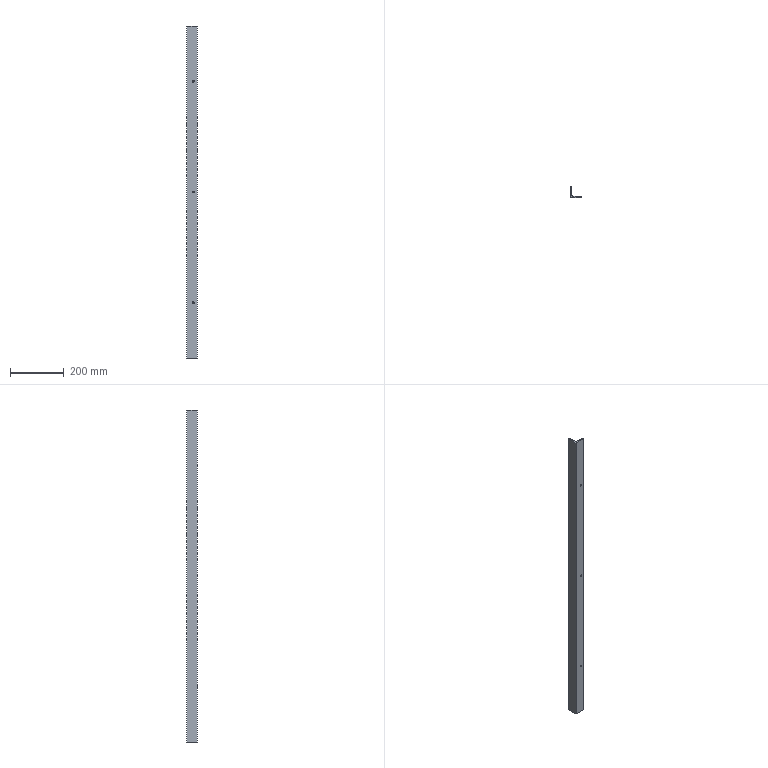Part | SolidWorks | features Extrusion 1, HoleWzd 1, LPattern 1 | 1 solid | 17 faces | box 40 x 40 x 1230 mm | volume 378926 mm3 | cylinder 9 | plane 8 | commonest cylinder face diameters 6 x6 0.02 x2 9 x1
STEP:
#1=CARTESIAN_POINT('',(25.,4.,1028.));
#2=VERTEX_POINT('',#1);
#3=CARTESIAN_POINT('',(25.,4.,1022.));
#4=VERTEX_POINT('',#3);
#5=CARTESIAN_POINT('',(25.,4.,1025.));
#6=DIRECTION('',(0.,-1.,0.));
#7=DIRECTION('',(1.,0.,0.));
#8=AXIS2_PLACEMENT_3D('',#5,#6,#7);
#9=CIRCLE('',#8,3.);
#10=EDGE_CURVE('',#2,#4,#9,.T.);
#11=ORIENTED_EDGE('',*,*,#10,.F.);
#12=CARTESIAN_POINT('',(25.,0.,1028.));
#13=VERTEX_POINT('',#12);
#14=CARTESIAN_POINT('',(25.,0.,1028.));
#15=DIRECTION('',(0.,-1.,0.));
#16=VECTOR('',#15,1000.);
#17=LINE('',#14,#16);
#18=EDGE_CURVE('',#2,#13,#17,.T.);
#19=ORIENTED_EDGE('',*,*,#18,.T.);
#20=CARTESIAN_POINT('',(25.,0.,1022.));
#21=VERTEX_POINT('',#20);
#22=CARTESIAN_POINT('',(25.,0.,1025.));
#23=DIRECTION('',(0.,-1.,0.));
#24=DIRECTION('',(0.,0.,-1.));
#25=AXIS2_PLACEMENT_3D('',#22,#23,#24);
#26=CIRCLE('',#25,3.);
#27=EDGE_CURVE('',#13,#21,#26,.T.);
#28=ORIENTED_EDGE('',*,*,#27,.T.);
#29=CARTESIAN_POINT('',(25.,0.,1022.));
#30=DIRECTION('',(0.,-1.,0.));
#31=VECTOR('',#30,1000.);
#32=LINE('',#29,#31);
#33=EDGE_CURVE('',#4,#21,#32,.T.);
#34=ORIENTED_EDGE('',*,*,#33,.F.);
#35=EDGE_LOOP('',(#11,#19,#28,#34));
#36=FACE_OUTER_BOUND('',#35,.T.);
#37=CARTESIAN_POINT('',(25.,0.,1025.));
#38=DIRECTION('',(0.,-1.,0.));
#39=DIRECTION('',(0.,0.,-1.));
#40=AXIS2_PLACEMENT_3D('',#37,#38,#39);
#41=CYLINDRICAL_SURFACE('',#40,3.);
#42=ADVANCED_FACE('',(#36),#41,.F.);
#43=CARTESIAN_POINT('',(25.,4.,618.));
#44=VERTEX_POINT('',#43);
#45=CARTESIAN_POINT('',(25.,4.,612.));
#46=VERTEX_POINT('',#45);
#47=CARTESIAN_POINT('',(25.,4.,615.));
#48=DIRECTION('',(0.,-1.,0.));
#49=DIRECTION('',(1.,0.,0.));
#50=AXIS2_PLACEMENT_3D('',#47,#48,#49);
#51=CIRCLE('',#50,3.);
#52=EDGE_CURVE('',#44,#46,#51,.T.);
#53=ORIENTED_EDGE('',*,*,#52,.F.);
#54=CARTESIAN_POINT('',(25.,0.,618.));
#55=VERTEX_POINT('',#54);
#56=CARTESIAN_POINT('',(25.,0.,618.));
#57=DIRECTION('',(0.,-1.,0.));
#58=VECTOR('',#57,1000.);
#59=LINE('',#56,#58);
#60=EDGE_CURVE('',#44,#55,#59,.T.);
#61=ORIENTED_EDGE('',*,*,#60,.T.);
#62=CARTESIAN_POINT('',(25.,0.,612.));
#63=VERTEX_POINT('',#62);
#64=CARTESIAN_POINT('',(25.,0.,615.));
#65=DIRECTION('',(0.,-1.,0.));
#66=DIRECTION('',(0.,0.,-1.));
#67=AXIS2_PLACEMENT_3D('',#64,#65,#66);
#68=CIRCLE('',#67,3.);
#69=EDGE_CURVE('',#55,#63,#68,.T.);
#70=ORIENTED_EDGE('',*,*,#69,.T.);
#71=CARTESIAN_POINT('',(25.,0.,612.));
#72=DIRECTION('',(0.,-1.,0.));
#73=VECTOR('',#72,1000.);
#74=LINE('',#71,#73);
#75=EDGE_CURVE('',#46,#63,#74,.T.);
#76=ORIENTED_EDGE('',*,*,#75,.F.);
#77=EDGE_LOOP('',(#53,#61,#70,#76));
#78=FACE_OUTER_BOUND('',#77,.T.);
#79=CARTESIAN_POINT('',(25.,0.,615.));
#80=DIRECTION('',(0.,-1.,0.));
#81=DIRECTION('',(0.,0.,-1.));
#82=AXIS2_PLACEMENT_3D('',#79,#80,#81);
#83=CYLINDRICAL_SURFACE('',#82,3.);
#84=ADVANCED_FACE('',(#78),#83,.F.);
#85=CARTESIAN_POINT('',(25.,4.,208.));
#86=VERTEX_POINT('',#85);
#87=CARTESIAN_POINT('',(25.,4.,202.));
#88=VERTEX_POINT('',#87);
#89=CARTESIAN_POINT('',(25.,4.,205.));
#90=DIRECTION('',(0.,-1.,0.));
#91=DIRECTION('',(1.,0.,0.));
#92=AXIS2_PLACEMENT_3D('',#89,#90,#91);
#93=CIRCLE('',#92,3.);
#94=EDGE_CURVE('',#86,#88,#93,.T.);
#95=ORIENTED_EDGE('',*,*,#94,.F.);
#96=CARTESIAN_POINT('',(25.,0.,208.));
#97=VERTEX_POINT('',#96);
#98=CARTESIAN_POINT('',(25.,0.,208.));
#99=DIRECTION('',(0.,-1.,0.));
#100=VECTOR('',#99,1000.);
#101=LINE('',#98,#100);
#102=EDGE_CURVE('',#86,#97,#101,.T.);
#103=ORIENTED_EDGE('',*,*,#102,.T.);
#104=CARTESIAN_POINT('',(25.,0.,202.));
#105=VERTEX_POINT('',#104);
#106=CARTESIAN_POINT('',(25.,0.,205.));
#107=DIRECTION('',(0.,-1.,0.));
#108=DIRECTION('',(0.,0.,-1.));
#109=AXIS2_PLACEMENT_3D('',#106,#107,#108);
#110=CIRCLE('',#109,3.);
#111=EDGE_CURVE('',#97,#105,#110,.T.);
#112=ORIENTED_EDGE('',*,*,#111,.T.);
#113=CARTESIAN_POINT('',(25.,0.,202.));
#114=DIRECTION('',(0.,-1.,0.));
#115=VECTOR('',#114,1000.);
#116=LINE('',#113,#115);
#117=EDGE_CURVE('',#88,#105,#116,.T.);
#118=ORIENTED_EDGE('',*,*,#117,.F.);
#119=EDGE_LOOP('',(#95,#103,#112,#118));
#120=FACE_OUTER_BOUND('',#119,.T.);
#121=CARTESIAN_POINT('',(25.,0.,205.));
#122=DIRECTION('',(0.,-1.,0.));
#123=DIRECTION('',(0.,0.,-1.));
#124=AXIS2_PLACEMENT_3D('',#121,#122,#123);
#125=CYLINDRICAL_SURFACE('',#124,3.);
#126=ADVANCED_FACE('',(#120),#125,.F.);
#127=CARTESIAN_POINT('',(25.,0.,615.));
#128=DIRECTION('',(0.,-1.,0.));
#129=DIRECTION('',(0.,0.,-1.));
#130=AXIS2_PLACEMENT_3D('',#127,#128,#129);
#131=CIRCLE('',#130,3.);
#132=EDGE_CURVE('',#63,#55,#131,.T.);
#133=ORIENTED_EDGE('',*,*,#132,.F.);
#134=ORIENTED_EDGE('',*,*,#69,.F.);
#135=EDGE_LOOP('',(#133,#134));
#136=FACE_BOUND('',#135,.T.);
#137=CARTESIAN_POINT('',(25.,0.,205.));
#138=DIRECTION('',(0.,-1.,0.));
#139=DIRECTION('',(0.,0.,-1.));
#140=AXIS2_PLACEMENT_3D('',#137,#138,#139);
#141=CIRCLE('',#140,3.);
#142=EDGE_CURVE('',#105,#97,#141,.T.);
#143=ORIENTED_EDGE('',*,*,#142,.F.);
#144=ORIENTED_EDGE('',*,*,#111,.F.);
#145=EDGE_LOOP('',(#143,#144));
#146=FACE_BOUND('',#145,.T.);
#147=CARTESIAN_POINT('',(0.,0.,0.));
#148=VERTEX_POINT('',#147);
#149=CARTESIAN_POINT('',(40.,0.,0.));
#150=VERTEX_POINT('',#149);
#151=CARTESIAN_POINT('',(40.,0.,0.));
#152=DIRECTION('',(1.,0.,0.));
#153=VECTOR('',#152,1000.);
#154=LINE('',#151,#153);
#155=EDGE_CURVE('',#148,#150,#154,.T.);
#156=ORIENTED_EDGE('',*,*,#155,.T.);
#157=CARTESIAN_POINT('',(40.,0.,1230.));
#158=VERTEX_POINT('',#157);
#159=CARTESIAN_POINT('',(40.,0.,1230.));
#160=DIRECTION('',(0.,0.,-1.));
#161=VECTOR('',#160,1000.);
#162=LINE('',#159,#161);
#163=EDGE_CURVE('',#158,#150,#162,.T.);
#164=ORIENTED_EDGE('',*,*,#163,.F.);
#165=CARTESIAN_POINT('',(0.,0.,1230.));
#166=VERTEX_POINT('',#165);
#167=CARTESIAN_POINT('',(40.,0.,1230.));
#168=DIRECTION('',(1.,0.,0.));
#169=VECTOR('',#168,1000.);
#170=LINE('',#167,#169);
#171=EDGE_CURVE('',#166,#158,#170,.T.);
#172=ORIENTED_EDGE('',*,*,#171,.F.);
#173=CARTESIAN_POINT('',(0.,0.,1230.));
#174=DIRECTION('',(0.,0.,-1.));
#175=VECTOR('',#174,1000.);
#176=LINE('',#173,#175);
#177=EDGE_CURVE('',#166,#148,#176,.T.);
#178=ORIENTED_EDGE('',*,*,#177,.T.);
#179=EDGE_LOOP('',(#156,#164,#172,#178));
#180=FACE_OUTER_BOUND('',#179,.T.);
#181=CARTESIAN_POINT('',(25.,0.,1025.));
#182=DIRECTION('',(0.,-1.,0.));
#183=DIRECTION('',(0.,0.,-1.));
#184=AXIS2_PLACEMENT_3D('',#181,#182,#183);
#185=CIRCLE('',#184,3.);
#186=EDGE_CURVE('',#21,#13,#185,.T.);
#187=ORIENTED_EDGE('',*,*,#186,.F.);
#188=ORIENTED_EDGE('',*,*,#27,.F.);
#189=EDGE_LOOP('',(#187,#188));
#190=FACE_BOUND('',#189,.T.);
#191=CARTESIAN_POINT('',(40.,0.,1230.));
#192=DIRECTION('',(0.,1.,0.));
#193=DIRECTION('',(-1.,0.,0.));
#194=AXIS2_PLACEMENT_3D('',#191,#192,#193);
#195=PLANE('',#194);
#196=ADVANCED_FACE('',(#136,#146,#180,#190),#195,.F.);
#197=CARTESIAN_POINT('',(40.,3.99,0.));
#198=VERTEX_POINT('',#197);
#199=CARTESIAN_POINT('',(40.,3.99,0.));
#200=DIRECTION('',(0.,1.,0.));
#201=VECTOR('',#200,1000.);
#202=LINE('',#199,#201);
#203=EDGE_CURVE('',#150,#198,#202,.T.);
#204=ORIENTED_EDGE('',*,*,#203,.T.);
#205=CARTESIAN_POINT('',(40.,3.99,1230.));
#206=VERTEX_POINT('',#205);
#207=CARTESIAN_POINT('',(40.,3.99,1230.));
#208=DIRECTION('',(0.,0.,-1.));
#209=VECTOR('',#208,1000.);
#210=LINE('',#207,#209);
#211=EDGE_CURVE('',#206,#198,#210,.T.);
#212=ORIENTED_EDGE('',*,*,#211,.F.);
#213=CARTESIAN_POINT('',(40.,3.99,1230.));
#214=DIRECTION('',(0.,1.,0.));
#215=VECTOR('',#214,1000.);
#216=LINE('',#213,#215);
#217=EDGE_CURVE('',#158,#206,#216,.T.);
#218=ORIENTED_EDGE('',*,*,#217,.F.);
#219=ORIENTED_EDGE('',*,*,#163,.T.);
#220=EDGE_LOOP('',(#204,#212,#218,#219));
#221=FACE_OUTER_BOUND('',#220,.T.);
#222=CARTESIAN_POINT('',(40.,3.99,1230.));
#223=DIRECTION('',(-1.,0.,0.));
#224=DIRECTION('',(0.,0.,1.));
#225=AXIS2_PLACEMENT_3D('',#222,#223,#224);
#226=PLANE('',#225);
#227=ADVANCED_FACE('',(#221),#226,.F.);
#228=CARTESIAN_POINT('',(39.99,4.,0.));
#229=VERTEX_POINT('',#228);
#230=CARTESIAN_POINT('',(39.99,3.99,0.));
#231=DIRECTION('',(0.,0.,1.));
#232=DIRECTION('',(1.,0.,0.));
#233=AXIS2_PLACEMENT_3D('',#230,#231,#232);
#234=CIRCLE('',#233,0.01);
#235=EDGE_CURVE('',#198,#229,#234,.T.);
#236=ORIENTED_EDGE('',*,*,#235,.T.);
#237=CARTESIAN_POINT('',(39.99,4.,1230.));
#238=VERTEX_POINT('',#237);
#239=CARTESIAN_POINT('',(39.99,4.,1230.));
#240=DIRECTION('',(0.,0.,-1.));
#241=VECTOR('',#240,1000.);
#242=LINE('',#239,#241);
#243=EDGE_CURVE('',#238,#229,#242,.T.);
#244=ORIENTED_EDGE('',*,*,#243,.F.);
#245=CARTESIAN_POINT('',(39.99,3.99,1230.));
#246=DIRECTION('',(0.,0.,1.));
#247=DIRECTION('',(1.,0.,0.));
#248=AXIS2_PLACEMENT_3D('',#245,#246,#247);
#249=CIRCLE('',#248,0.01);
#250=EDGE_CURVE('',#206,#238,#249,.T.);
#251=ORIENTED_EDGE('',*,*,#250,.F.);
#252=ORIENTED_EDGE('',*,*,#211,.T.);
#253=EDGE_LOOP('',(#236,#244,#251,#252));
#254=FACE_OUTER_BOUND('',#253,.T.);
#255=CARTESIAN_POINT('',(39.99,3.99,1230.));
#256=DIRECTION('',(0.,0.,-1.));
#257=DIRECTION('',(-1.,0.,0.));
#258=AXIS2_PLACEMENT_3D('',#255,#256,#257);
#259=CYLINDRICAL_SURFACE('',#258,0.01);
#260=ADVANCED_FACE('',(#254),#259,.T.);
#261=CARTESIAN_POINT('',(25.,4.,615.));
#262=DIRECTION('',(0.,-1.,0.));
#263=DIRECTION('',(1.,0.,0.));
#264=AXIS2_PLACEMENT_3D('',#261,#262,#263);
#265=CIRCLE('',#264,3.);
#266=EDGE_CURVE('',#46,#44,#265,.T.);
#267=ORIENTED_EDGE('',*,*,#266,.T.);
#268=ORIENTED_EDGE('',*,*,#52,.T.);
#269=EDGE_LOOP('',(#267,#268));
#270=FACE_BOUND('',#269,.T.);
#271=CARTESIAN_POINT('',(25.,4.,205.));
#272=DIRECTION('',(0.,-1.,0.));
#273=DIRECTION('',(1.,0.,0.));
#274=AXIS2_PLACEMENT_3D('',#271,#272,#273);
#275=CIRCLE('',#274,3.);
#276=EDGE_CURVE('',#88,#86,#275,.T.);
#277=ORIENTED_EDGE('',*,*,#276,.T.);
#278=ORIENTED_EDGE('',*,*,#94,.T.);
#279=EDGE_LOOP('',(#277,#278));
#280=FACE_BOUND('',#279,.T.);
#281=CARTESIAN_POINT('',(8.5,4.,0.));
#282=VERTEX_POINT('',#281);
#283=CARTESIAN_POINT('',(8.5,4.,0.));
#284=DIRECTION('',(-1.,0.,0.));
#285=VECTOR('',#284,1000.);
#286=LINE('',#283,#285);
#287=EDGE_CURVE('',#229,#282,#286,.T.);
#288=ORIENTED_EDGE('',*,*,#287,.T.);
#289=CARTESIAN_POINT('',(8.5,4.,1230.));
#290=VERTEX_POINT('',#289);
#291=CARTESIAN_POINT('',(8.5,4.,1230.));
#292=DIRECTION('',(0.,0.,-1.));
#293=VECTOR('',#292,1000.);
#294=LINE('',#291,#293);
#295=EDGE_CURVE('',#290,#282,#294,.T.);
#296=ORIENTED_EDGE('',*,*,#295,.F.);
#297=CARTESIAN_POINT('',(8.5,4.,1230.));
#298=DIRECTION('',(-1.,0.,0.));
#299=VECTOR('',#298,1000.);
#300=LINE('',#297,#299);
#301=EDGE_CURVE('',#238,#290,#300,.T.);
#302=ORIENTED_EDGE('',*,*,#301,.F.);
#303=ORIENTED_EDGE('',*,*,#243,.T.);
#304=EDGE_LOOP('',(#288,#296,#302,#303));
#305=FACE_OUTER_BOUND('',#304,.T.);
#306=CARTESIAN_POINT('',(25.,4.,1025.));
#307=DIRECTION('',(0.,-1.,0.));
#308=DIRECTION('',(1.,0.,0.));
#309=AXIS2_PLACEMENT_3D('',#306,#307,#308);
#310=CIRCLE('',#309,3.);
#311=EDGE_CURVE('',#4,#2,#310,.T.);
#312=ORIENTED_EDGE('',*,*,#311,.T.);
#313=ORIENTED_EDGE('',*,*,#10,.T.);
#314=EDGE_LOOP('',(#312,#313));
#315=FACE_BOUND('',#314,.T.);
#316=CARTESIAN_POINT('',(8.5,4.,1230.));
#317=DIRECTION('',(0.,-1.,0.));
#318=DIRECTION('',(1.,0.,0.));
#319=AXIS2_PLACEMENT_3D('',#316,#317,#318);
#320=PLANE('',#319);
#321=ADVANCED_FACE('',(#270,#280,#305,#315),#320,.F.);
#322=CARTESIAN_POINT('',(4.,8.5,0.));
#323=VERTEX_POINT('',#322);
#324=CARTESIAN_POINT('',(8.5,8.5,0.));
#325=DIRECTION('',(0.,0.,-1.));
#326=DIRECTION('',(-1.,0.,0.));
#327=AXIS2_PLACEMENT_3D('',#324,#325,#326);
#328=CIRCLE('',#327,4.5);
#329=EDGE_CURVE('',#282,#323,#328,.T.);
#330=ORIENTED_EDGE('',*,*,#329,.T.);
#331=CARTESIAN_POINT('',(4.,8.5,1230.));
#332=VERTEX_POINT('',#331);
#333=CARTESIAN_POINT('',(4.,8.5,1230.));
#334=DIRECTION('',(0.,0.,-1.));
#335=VECTOR('',#334,1000.);
#336=LINE('',#333,#335);
#337=EDGE_CURVE('',#332,#323,#336,.T.);
#338=ORIENTED_EDGE('',*,*,#337,.F.);
#339=CARTESIAN_POINT('',(8.5,8.5,1230.));
#340=DIRECTION('',(0.,0.,-1.));
#341=DIRECTION('',(-1.,0.,0.));
#342=AXIS2_PLACEMENT_3D('',#339,#340,#341);
#343=CIRCLE('',#342,4.5);
#344=EDGE_CURVE('',#290,#332,#343,.T.);
#345=ORIENTED_EDGE('',*,*,#344,.F.);
#346=ORIENTED_EDGE('',*,*,#295,.T.);
#347=EDGE_LOOP('',(#330,#338,#345,#346));
#348=FACE_OUTER_BOUND('',#347,.T.);
#349=CARTESIAN_POINT('',(8.5,8.5,1230.));
#350=DIRECTION('',(0.,0.,-1.));
#351=DIRECTION('',(-1.,0.,0.));
#352=AXIS2_PLACEMENT_3D('',#349,#350,#351);
#353=CYLINDRICAL_SURFACE('',#352,4.5);
#354=ADVANCED_FACE('',(#348),#353,.F.);
#355=CARTESIAN_POINT('',(4.,39.99,0.));
#356=VERTEX_POINT('',#355);
#357=CARTESIAN_POINT('',(4.,39.99,0.));
#358=DIRECTION('',(0.,1.,0.));
#359=VECTOR('',#358,1000.);
#360=LINE('',#357,#359);
#361=EDGE_CURVE('',#323,#356,#360,.T.);
#362=ORIENTED_EDGE('',*,*,#361,.T.);
#363=CARTESIAN_POINT('',(4.,39.99,1230.));
#364=VERTEX_POINT('',#363);
#365=CARTESIAN_POINT('',(4.,39.99,1230.));
#366=DIRECTION('',(0.,0.,-1.));
#367=VECTOR('',#366,1000.);
#368=LINE('',#365,#367);
#369=EDGE_CURVE('',#364,#356,#368,.T.);
#370=ORIENTED_EDGE('',*,*,#369,.F.);
#371=CARTESIAN_POINT('',(4.,39.99,1230.));
#372=DIRECTION('',(0.,1.,0.));
#373=VECTOR('',#372,1000.);
#374=LINE('',#371,#373);
#375=EDGE_CURVE('',#332,#364,#374,.T.);
#376=ORIENTED_EDGE('',*,*,#375,.F.);
#377=ORIENTED_EDGE('',*,*,#337,.T.);
#378=EDGE_LOOP('',(#362,#370,#376,#377));
#379=FACE_OUTER_BOUND('',#378,.T.);
#380=CARTESIAN_POINT('',(4.,39.99,1230.));
#381=DIRECTION('',(-1.,0.,0.));
#382=DIRECTION('',(0.,-1.,0.));
#383=AXIS2_PLACEMENT_3D('',#380,#381,#382);
#384=PLANE('',#383);
#385=ADVANCED_FACE('',(#379),#384,.F.);
#386=CARTESIAN_POINT('',(3.99,40.,0.));
#387=VERTEX_POINT('',#386);
#388=CARTESIAN_POINT('',(3.99,39.99,0.));
#389=DIRECTION('',(0.,0.,1.));
#390=DIRECTION('',(1.,0.,0.));
#391=AXIS2_PLACEMENT_3D('',#388,#389,#390);
#392=CIRCLE('',#391,0.01);
#393=EDGE_CURVE('',#356,#387,#392,.T.);
#394=ORIENTED_EDGE('',*,*,#393,.T.);
#395=CARTESIAN_POINT('',(3.99,40.,1230.));
#396=VERTEX_POINT('',#395);
#397=CARTESIAN_POINT('',(3.99,40.,1230.));
#398=DIRECTION('',(0.,0.,-1.));
#399=VECTOR('',#398,1000.);
#400=LINE('',#397,#399);
#401=EDGE_CURVE('',#396,#387,#400,.T.);
#402=ORIENTED_EDGE('',*,*,#401,.F.);
#403=CARTESIAN_POINT('',(3.99,39.99,1230.));
#404=DIRECTION('',(0.,0.,1.));
#405=DIRECTION('',(1.,0.,0.));
#406=AXIS2_PLACEMENT_3D('',#403,#404,#405);
#407=CIRCLE('',#406,0.01);
#408=EDGE_CURVE('',#364,#396,#407,.T.);
#409=ORIENTED_EDGE('',*,*,#408,.F.);
#410=ORIENTED_EDGE('',*,*,#369,.T.);
#411=EDGE_LOOP('',(#394,#402,#409,#410));
#412=FACE_OUTER_BOUND('',#411,.T.);
#413=CARTESIAN_POINT('',(3.99,39.99,1230.));
#414=DIRECTION('',(0.,0.,-1.));
#415=DIRECTION('',(-1.,0.,0.));
#416=AXIS2_PLACEMENT_3D('',#413,#414,#415);
#417=CYLINDRICAL_SURFACE('',#416,0.01);
#418=ADVANCED_FACE('',(#412),#417,.T.);
#419=CARTESIAN_POINT('',(0.,40.,0.));
#420=VERTEX_POINT('',#419);
#421=CARTESIAN_POINT('',(0.,40.,0.));
#422=DIRECTION('',(-1.,0.,0.));
#423=VECTOR('',#422,1000.);
#424=LINE('',#421,#423);
#425=EDGE_CURVE('',#387,#420,#424,.T.);
#426=ORIENTED_EDGE('',*,*,#425,.T.);
#427=CARTESIAN_POINT('',(0.,40.,1230.));
#428=VERTEX_POINT('',#427);
#429=CARTESIAN_POINT('',(0.,40.,1230.));
#430=DIRECTION('',(0.,0.,-1.));
#431=VECTOR('',#430,1000.);
#432=LINE('',#429,#431);
#433=EDGE_CURVE('',#428,#420,#432,.T.);
#434=ORIENTED_EDGE('',*,*,#433,.F.);
#435=CARTESIAN_POINT('',(0.,40.,1230.));
#436=DIRECTION('',(-1.,0.,0.));
#437=VECTOR('',#436,1000.);
#438=LINE('',#435,#437);
#439=EDGE_CURVE('',#396,#428,#438,.T.);
#440=ORIENTED_EDGE('',*,*,#439,.F.);
#441=ORIENTED_EDGE('',*,*,#401,.T.);
#442=EDGE_LOOP('',(#426,#434,#440,#441));
#443=FACE_OUTER_BOUND('',#442,.T.);
#444=CARTESIAN_POINT('',(0.,40.,1230.));
#445=DIRECTION('',(0.,-1.,0.));
#446=DIRECTION('',(0.,0.,-1.));
#447=AXIS2_PLACEMENT_3D('',#444,#445,#446);
#448=PLANE('',#447);
#449=ADVANCED_FACE('',(#443),#448,.F.);
#450=CARTESIAN_POINT('',(0.,0.,0.));
#451=DIRECTION('',(0.,-1.,0.));
#452=VECTOR('',#451,1000.);
#453=LINE('',#450,#452);
#454=EDGE_CURVE('',#420,#148,#453,.T.);
#455=ORIENTED_EDGE('',*,*,#454,.T.);
#456=ORIENTED_EDGE('',*,*,#177,.F.);
#457=CARTESIAN_POINT('',(0.,0.,1230.));
#458=DIRECTION('',(0.,-1.,0.));
#459=VECTOR('',#458,1000.);
#460=LINE('',#457,#459);
#461=EDGE_CURVE('',#428,#166,#460,.T.);
#462=ORIENTED_EDGE('',*,*,#461,.F.);
#463=ORIENTED_EDGE('',*,*,#433,.T.);
#464=EDGE_LOOP('',(#455,#456,#462,#463));
#465=FACE_OUTER_BOUND('',#464,.T.);
#466=CARTESIAN_POINT('',(0.,0.,1230.));
#467=DIRECTION('',(1.,0.,0.));
#468=DIRECTION('',(0.,0.,-1.));
#469=AXIS2_PLACEMENT_3D('',#466,#467,#468);
#470=PLANE('',#469);
#471=ADVANCED_FACE('',(#465),#470,.F.);
#472=ORIENTED_EDGE('',*,*,#171,.T.);
#473=ORIENTED_EDGE('',*,*,#217,.T.);
#474=ORIENTED_EDGE('',*,*,#250,.T.);
#475=ORIENTED_EDGE('',*,*,#301,.T.);
#476=ORIENTED_EDGE('',*,*,#344,.T.);
#477=ORIENTED_EDGE('',*,*,#375,.T.);
#478=ORIENTED_EDGE('',*,*,#408,.T.);
#479=ORIENTED_EDGE('',*,*,#439,.T.);
#480=ORIENTED_EDGE('',*,*,#461,.T.);
#481=EDGE_LOOP('',(#472,#473,#474,#475,#476,#477,#478,#479,#480));
#482=FACE_OUTER_BOUND('',#481,.T.);
#483=CARTESIAN_POINT('',(3.99,39.99,1230.));
#484=DIRECTION('',(0.,0.,1.));
#485=DIRECTION('',(1.,0.,0.));
#486=AXIS2_PLACEMENT_3D('',#483,#484,#485);
#487=PLANE('',#486);
#488=ADVANCED_FACE('',(#482),#487,.T.);
#489=ORIENTED_EDGE('',*,*,#155,.F.);
#490=ORIENTED_EDGE('',*,*,#454,.F.);
#491=ORIENTED_EDGE('',*,*,#425,.F.);
#492=ORIENTED_EDGE('',*,*,#393,.F.);
#493=ORIENTED_EDGE('',*,*,#361,.F.);
#494=ORIENTED_EDGE('',*,*,#329,.F.);
#495=ORIENTED_EDGE('',*,*,#287,.F.);
#496=ORIENTED_EDGE('',*,*,#235,.F.);
#497=ORIENTED_EDGE('',*,*,#203,.F.);
#498=EDGE_LOOP('',(#489,#490,#491,#492,#493,#494,#495,#496,#497));
#499=FACE_OUTER_BOUND('',#498,.T.);
#500=CARTESIAN_POINT('',(3.99,39.99,0.));
#501=DIRECTION('',(0.,0.,1.));
#502=DIRECTION('',(1.,0.,0.));
#503=AXIS2_PLACEMENT_3D('',#500,#501,#502);
#504=PLANE('',#503);
#505=ADVANCED_FACE('',(#499),#504,.F.);
#506=ORIENTED_EDGE('',*,*,#102,.F.);
#507=ORIENTED_EDGE('',*,*,#276,.F.);
#508=ORIENTED_EDGE('',*,*,#117,.T.);
#509=ORIENTED_EDGE('',*,*,#142,.T.);
#510=EDGE_LOOP('',(#506,#507,#508,#509));
#511=FACE_OUTER_BOUND('',#510,.T.);
#512=CARTESIAN_POINT('',(25.,0.,205.));
#513=DIRECTION('',(0.,-1.,0.));
#514=DIRECTION('',(0.,0.,-1.));
#515=AXIS2_PLACEMENT_3D('',#512,#513,#514);
#516=CYLINDRICAL_SURFACE('',#515,3.);
#517=ADVANCED_FACE('',(#511),#516,.F.);
#518=ORIENTED_EDGE('',*,*,#60,.F.);
#519=ORIENTED_EDGE('',*,*,#266,.F.);
#520=ORIENTED_EDGE('',*,*,#75,.T.);
#521=ORIENTED_EDGE('',*,*,#132,.T.);
#522=EDGE_LOOP('',(#518,#519,#520,#521));
#523=FACE_OUTER_BOUND('',#522,.T.);
#524=CARTESIAN_POINT('',(25.,0.,615.));
#525=DIRECTION('',(0.,-1.,0.));
#526=DIRECTION('',(0.,0.,-1.));
#527=AXIS2_PLACEMENT_3D('',#524,#525,#526);
#528=CYLINDRICAL_SURFACE('',#527,3.);
#529=ADVANCED_FACE('',(#523),#528,.F.);
#530=ORIENTED_EDGE('',*,*,#18,.F.);
#531=ORIENTED_EDGE('',*,*,#311,.F.);
#532=ORIENTED_EDGE('',*,*,#33,.T.);
#533=ORIENTED_EDGE('',*,*,#186,.T.);
#534=EDGE_LOOP('',(#530,#531,#532,#533));
#535=FACE_OUTER_BOUND('',#534,.T.);
#536=CARTESIAN_POINT('',(25.,0.,1025.));
#537=DIRECTION('',(0.,-1.,0.));
#538=DIRECTION('',(0.,0.,-1.));
#539=AXIS2_PLACEMENT_3D('',#536,#537,#538);
#540=CYLINDRICAL_SURFACE('',#539,3.);
#541=ADVANCED_FACE('',(#535),#540,.F.);
#542=CLOSED_SHELL('',(#42,#84,#126,#196,#227,#260,#321,#354,#385,#418,#449,#471,#488,#505,#517,#529,#541));
#543=MANIFOLD_SOLID_BREP('',#542);
#544=CARTESIAN_POINT('',(0.,0.,0.));
#545=DIRECTION('',(0.,0.,1.));
#546=DIRECTION('',(1.,0.,0.));
#547=AXIS2_PLACEMENT_3D('',#544,#545,#546);
#548=(LENGTH_UNIT()NAMED_UNIT(*)SI_UNIT(.MILLI.,.METRE.));
#549=UNCERTAINTY_MEASURE_WITH_UNIT(LENGTH_MEASURE(0.00001),#548,'','');
#550=(NAMED_UNIT(*)PLANE_ANGLE_UNIT()SI_UNIT($,.RADIAN.));
#551=(NAMED_UNIT(*)SI_UNIT($,.STERADIAN.)SOLID_ANGLE_UNIT());
#552=(GEOMETRIC_REPRESENTATION_CONTEXT(3)GLOBAL_UNCERTAINTY_ASSIGNED_CONTEXT((#549))GLOBAL_UNIT_ASSIGNED_CONTEXT((#548,#550,#551))REPRESENTATION_CONTEXT('',''));
#553=ADVANCED_BREP_SHAPE_REPRESENTATION('',(#543,#547),#552);